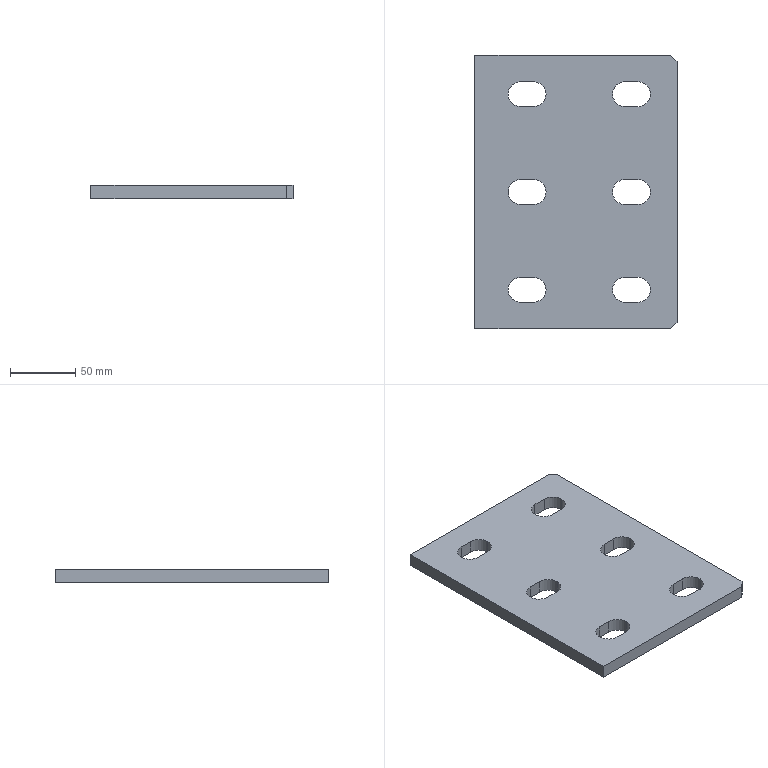Part | STEP file | 立柱翼Plate筋Plate-250 | 1 solid | 38 faces | box 155 x 210 x 10 mm | volume 296838 mm3 | plane 20 | cylinder 18 | commonest cylinder face diameters 19 x18